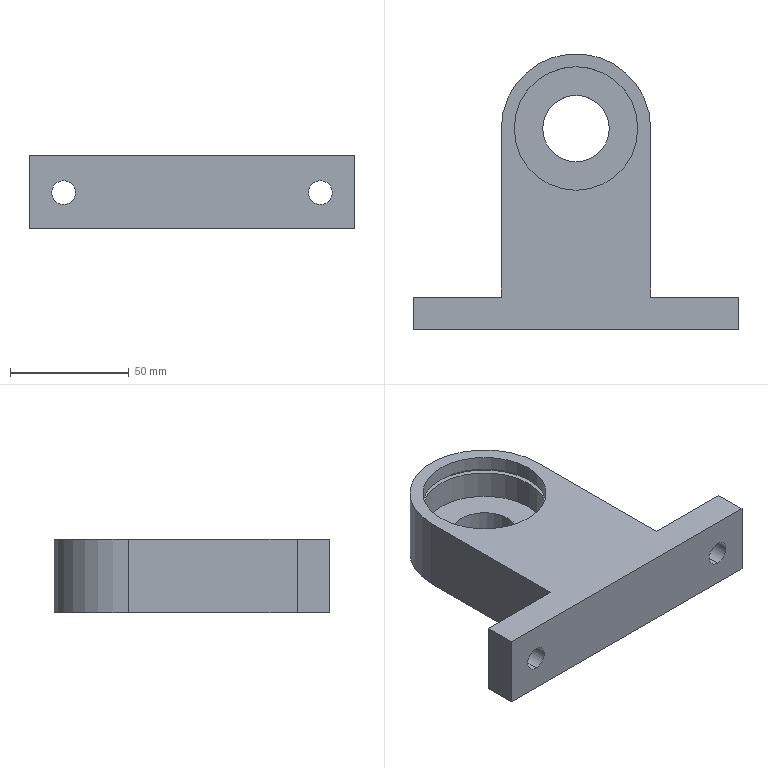Part | SolidWorks | features ICE 3, Cut 1, Extrusion 1 | 1 solid | 25 faces | box 137.013 x 116.006 x 31 mm | volume 192152 mm3 | cylinder 13 | plane 12 | commonest cylinder face diameters 10 x4 52 x4 28 x2 56.2 x2 62.794 x1
STEP:
#1=CARTESIAN_POINT('',(-28.1,0.,25.));
#2=VERTEX_POINT('',#1);
#3=CARTESIAN_POINT('',(28.1,0.,25.));
#4=VERTEX_POINT('',#3);
#5=CARTESIAN_POINT('',(0.,0.,25.));
#6=DIRECTION('',(0.,0.,1.));
#7=DIRECTION('',(1.,0.,0.));
#8=AXIS2_PLACEMENT_3D('',#5,#6,#7);
#9=CIRCLE('',#8,28.1);
#10=EDGE_CURVE('',#2,#4,#9,.T.);
#11=ORIENTED_EDGE('',*,*,#10,.T.);
#12=CARTESIAN_POINT('',(28.1,0.,23.));
#13=VERTEX_POINT('',#12);
#14=CARTESIAN_POINT('',(28.1,0.,25.));
#15=DIRECTION('',(0.,0.,-1.));
#16=VECTOR('',#15,1000.);
#17=LINE('',#14,#16);
#18=EDGE_CURVE('',#4,#13,#17,.T.);
#19=ORIENTED_EDGE('',*,*,#18,.T.);
#20=CARTESIAN_POINT('',(-28.1,0.,23.));
#21=VERTEX_POINT('',#20);
#22=CARTESIAN_POINT('',(0.,0.,23.));
#23=DIRECTION('',(0.,0.,1.));
#24=DIRECTION('',(1.,0.,0.));
#25=AXIS2_PLACEMENT_3D('',#22,#23,#24);
#26=CIRCLE('',#25,28.1);
#27=EDGE_CURVE('',#21,#13,#26,.T.);
#28=ORIENTED_EDGE('',*,*,#27,.F.);
#29=CARTESIAN_POINT('',(-28.1,0.,25.));
#30=DIRECTION('',(0.,0.,-1.));
#31=VECTOR('',#30,1000.);
#32=LINE('',#29,#31);
#33=EDGE_CURVE('',#2,#21,#32,.T.);
#34=ORIENTED_EDGE('',*,*,#33,.F.);
#35=EDGE_LOOP('',(#11,#19,#28,#34));
#36=FACE_OUTER_BOUND('',#35,.T.);
#37=CARTESIAN_POINT('',(0.,0.,25.));
#38=DIRECTION('',(0.,0.,-1.));
#39=DIRECTION('',(-1.,0.,0.));
#40=AXIS2_PLACEMENT_3D('',#37,#38,#39);
#41=CYLINDRICAL_SURFACE('',#40,28.1);
#42=ADVANCED_FACE('',(#36),#41,.F.);
#43=CARTESIAN_POINT('',(26.,0.,25.));
#44=VERTEX_POINT('',#43);
#45=CARTESIAN_POINT('',(-26.,0.,25.));
#46=VERTEX_POINT('',#45);
#47=CARTESIAN_POINT('',(0.,0.,25.));
#48=DIRECTION('',(0.,0.,-1.));
#49=DIRECTION('',(1.,0.,0.));
#50=AXIS2_PLACEMENT_3D('',#47,#48,#49);
#51=CIRCLE('',#50,26.);
#52=EDGE_CURVE('',#44,#46,#51,.T.);
#53=ORIENTED_EDGE('',*,*,#52,.T.);
#54=CARTESIAN_POINT('',(-26.,0.,31.));
#55=VERTEX_POINT('',#54);
#56=CARTESIAN_POINT('',(-26.,0.,11.));
#57=DIRECTION('',(0.,0.,1.));
#58=VECTOR('',#57,1000.);
#59=LINE('',#56,#58);
#60=EDGE_CURVE('',#46,#55,#59,.T.);
#61=ORIENTED_EDGE('',*,*,#60,.T.);
#62=CARTESIAN_POINT('',(26.,0.,31.));
#63=VERTEX_POINT('',#62);
#64=CARTESIAN_POINT('',(0.,0.,31.));
#65=DIRECTION('',(0.,0.,1.));
#66=DIRECTION('',(1.,0.,0.));
#67=AXIS2_PLACEMENT_3D('',#64,#65,#66);
#68=CIRCLE('',#67,26.);
#69=EDGE_CURVE('',#55,#63,#68,.T.);
#70=ORIENTED_EDGE('',*,*,#69,.T.);
#71=CARTESIAN_POINT('',(26.,0.,11.));
#72=DIRECTION('',(0.,0.,1.));
#73=VECTOR('',#72,1000.);
#74=LINE('',#71,#73);
#75=EDGE_CURVE('',#44,#63,#74,.T.);
#76=ORIENTED_EDGE('',*,*,#75,.F.);
#77=EDGE_LOOP('',(#53,#61,#70,#76));
#78=FACE_OUTER_BOUND('',#77,.T.);
#79=CARTESIAN_POINT('',(0.,0.,11.));
#80=DIRECTION('',(0.,0.,1.));
#81=DIRECTION('',(1.,0.,0.));
#82=AXIS2_PLACEMENT_3D('',#79,#80,#81);
#83=CYLINDRICAL_SURFACE('',#82,26.);
#84=ADVANCED_FACE('',(#78),#83,.F.);
#85=CARTESIAN_POINT('',(-54.,-84.609,20.251));
#86=VERTEX_POINT('',#85);
#87=CARTESIAN_POINT('',(-54.,-84.609,10.251));
#88=VERTEX_POINT('',#87);
#89=CARTESIAN_POINT('',(-54.,-84.609,15.251));
#90=DIRECTION('',(0.,-1.,0.));
#91=DIRECTION('',(0.,0.,1.));
#92=AXIS2_PLACEMENT_3D('',#89,#90,#91);
#93=CIRCLE('',#92,5.);
#94=EDGE_CURVE('',#86,#88,#93,.T.);
#95=ORIENTED_EDGE('',*,*,#94,.T.);
#96=CARTESIAN_POINT('',(-54.,-70.889,10.251));
#97=VERTEX_POINT('',#96);
#98=CARTESIAN_POINT('',(-54.,-101.889,10.251));
#99=DIRECTION('',(0.,1.,0.));
#100=VECTOR('',#99,1000.);
#101=LINE('',#98,#100);
#102=EDGE_CURVE('',#88,#97,#101,.T.);
#103=ORIENTED_EDGE('',*,*,#102,.T.);
#104=CARTESIAN_POINT('',(-54.,-70.889,20.251));
#105=VERTEX_POINT('',#104);
#106=CARTESIAN_POINT('',(-54.,-70.889,15.251));
#107=DIRECTION('',(0.,-1.,0.));
#108=DIRECTION('',(0.,0.,1.));
#109=AXIS2_PLACEMENT_3D('',#106,#107,#108);
#110=CIRCLE('',#109,5.);
#111=EDGE_CURVE('',#105,#97,#110,.T.);
#112=ORIENTED_EDGE('',*,*,#111,.F.);
#113=CARTESIAN_POINT('',(-54.,-101.889,20.251));
#114=DIRECTION('',(0.,1.,0.));
#115=VECTOR('',#114,1000.);
#116=LINE('',#113,#115);
#117=EDGE_CURVE('',#86,#105,#116,.T.);
#118=ORIENTED_EDGE('',*,*,#117,.F.);
#119=EDGE_LOOP('',(#95,#103,#112,#118));
#120=FACE_OUTER_BOUND('',#119,.T.);
#121=CARTESIAN_POINT('',(-54.,-101.889,15.251));
#122=DIRECTION('',(0.,1.,0.));
#123=DIRECTION('',(0.,0.,1.));
#124=AXIS2_PLACEMENT_3D('',#121,#122,#123);
#125=CYLINDRICAL_SURFACE('',#124,5.);
#126=ADVANCED_FACE('',(#120),#125,.F.);
#127=CARTESIAN_POINT('',(54.,-84.609,10.251));
#128=VERTEX_POINT('',#127);
#129=CARTESIAN_POINT('',(54.,-84.609,20.251));
#130=VERTEX_POINT('',#129);
#131=CARTESIAN_POINT('',(54.,-84.609,15.251));
#132=DIRECTION('',(0.,1.,0.));
#133=DIRECTION('',(0.,0.,1.));
#134=AXIS2_PLACEMENT_3D('',#131,#132,#133);
#135=CIRCLE('',#134,5.);
#136=EDGE_CURVE('',#128,#130,#135,.T.);
#137=ORIENTED_EDGE('',*,*,#136,.F.);
#138=CARTESIAN_POINT('',(54.,-70.889,10.251));
#139=VERTEX_POINT('',#138);
#140=CARTESIAN_POINT('',(54.,-101.889,10.251));
#141=DIRECTION('',(0.,1.,0.));
#142=VECTOR('',#141,1000.);
#143=LINE('',#140,#142);
#144=EDGE_CURVE('',#128,#139,#143,.T.);
#145=ORIENTED_EDGE('',*,*,#144,.T.);
#146=CARTESIAN_POINT('',(54.,-70.889,20.251));
#147=VERTEX_POINT('',#146);
#148=CARTESIAN_POINT('',(54.,-70.889,15.251));
#149=DIRECTION('',(0.,1.,0.));
#150=DIRECTION('',(0.,0.,1.));
#151=AXIS2_PLACEMENT_3D('',#148,#149,#150);
#152=CIRCLE('',#151,5.);
#153=EDGE_CURVE('',#139,#147,#152,.T.);
#154=ORIENTED_EDGE('',*,*,#153,.T.);
#155=CARTESIAN_POINT('',(54.,-101.889,20.251));
#156=DIRECTION('',(0.,1.,0.));
#157=VECTOR('',#156,1000.);
#158=LINE('',#155,#157);
#159=EDGE_CURVE('',#130,#147,#158,.T.);
#160=ORIENTED_EDGE('',*,*,#159,.F.);
#161=EDGE_LOOP('',(#137,#145,#154,#160));
#162=FACE_OUTER_BOUND('',#161,.T.);
#163=CARTESIAN_POINT('',(54.,-101.889,15.251));
#164=DIRECTION('',(0.,1.,0.));
#165=DIRECTION('',(0.,0.,1.));
#166=AXIS2_PLACEMENT_3D('',#163,#164,#165);
#167=CYLINDRICAL_SURFACE('',#166,5.);
#168=ADVANCED_FACE('',(#162),#167,.F.);
#169=CARTESIAN_POINT('',(14.,0.,11.));
#170=VERTEX_POINT('',#169);
#171=CARTESIAN_POINT('',(-14.,0.,11.));
#172=VERTEX_POINT('',#171);
#173=CARTESIAN_POINT('',(0.,0.,11.));
#174=DIRECTION('',(0.,0.,-1.));
#175=DIRECTION('',(1.,0.,0.));
#176=AXIS2_PLACEMENT_3D('',#173,#174,#175);
#177=CIRCLE('',#176,14.);
#178=EDGE_CURVE('',#170,#172,#177,.T.);
#179=ORIENTED_EDGE('',*,*,#178,.F.);
#180=CARTESIAN_POINT('',(14.,0.,0.));
#181=VERTEX_POINT('',#180);
#182=CARTESIAN_POINT('',(14.,0.,31.));
#183=DIRECTION('',(0.,0.,-1.));
#184=VECTOR('',#183,1000.);
#185=LINE('',#182,#184);
#186=EDGE_CURVE('',#170,#181,#185,.T.);
#187=ORIENTED_EDGE('',*,*,#186,.T.);
#188=CARTESIAN_POINT('',(-14.,0.,0.));
#189=VERTEX_POINT('',#188);
#190=CARTESIAN_POINT('',(0.,0.,0.));
#191=DIRECTION('',(0.,0.,-1.));
#192=DIRECTION('',(-1.,0.,0.));
#193=AXIS2_PLACEMENT_3D('',#190,#191,#192);
#194=CIRCLE('',#193,14.);
#195=EDGE_CURVE('',#181,#189,#194,.T.);
#196=ORIENTED_EDGE('',*,*,#195,.T.);
#197=CARTESIAN_POINT('',(-14.,0.,31.));
#198=DIRECTION('',(0.,0.,-1.));
#199=VECTOR('',#198,1000.);
#200=LINE('',#197,#199);
#201=EDGE_CURVE('',#172,#189,#200,.T.);
#202=ORIENTED_EDGE('',*,*,#201,.F.);
#203=EDGE_LOOP('',(#179,#187,#196,#202));
#204=FACE_OUTER_BOUND('',#203,.T.);
#205=CARTESIAN_POINT('',(0.,0.,31.));
#206=DIRECTION('',(0.,0.,-1.));
#207=DIRECTION('',(-1.,0.,0.));
#208=AXIS2_PLACEMENT_3D('',#205,#206,#207);
#209=CYLINDRICAL_SURFACE('',#208,14.);
#210=ADVANCED_FACE('',(#204),#209,.F.);
#211=CARTESIAN_POINT('',(-26.,0.,11.));
#212=VERTEX_POINT('',#211);
#213=CARTESIAN_POINT('',(26.,0.,11.));
#214=VERTEX_POINT('',#213);
#215=CARTESIAN_POINT('',(0.,0.,11.));
#216=DIRECTION('',(0.,0.,1.));
#217=DIRECTION('',(1.,0.,0.));
#218=AXIS2_PLACEMENT_3D('',#215,#216,#217);
#219=CIRCLE('',#218,26.);
#220=EDGE_CURVE('',#212,#214,#219,.T.);
#221=ORIENTED_EDGE('',*,*,#220,.F.);
#222=CARTESIAN_POINT('',(-26.,0.,23.));
#223=VERTEX_POINT('',#222);
#224=CARTESIAN_POINT('',(-26.,0.,11.));
#225=DIRECTION('',(0.,0.,1.));
#226=VECTOR('',#225,1000.);
#227=LINE('',#224,#226);
#228=EDGE_CURVE('',#212,#223,#227,.T.);
#229=ORIENTED_EDGE('',*,*,#228,.T.);
#230=CARTESIAN_POINT('',(26.,0.,23.));
#231=VERTEX_POINT('',#230);
#232=CARTESIAN_POINT('',(0.,0.,23.));
#233=DIRECTION('',(0.,0.,-1.));
#234=DIRECTION('',(1.,0.,0.));
#235=AXIS2_PLACEMENT_3D('',#232,#233,#234);
#236=CIRCLE('',#235,26.);
#237=EDGE_CURVE('',#231,#223,#236,.T.);
#238=ORIENTED_EDGE('',*,*,#237,.F.);
#239=CARTESIAN_POINT('',(26.,0.,11.));
#240=DIRECTION('',(0.,0.,1.));
#241=VECTOR('',#240,1000.);
#242=LINE('',#239,#241);
#243=EDGE_CURVE('',#214,#231,#242,.T.);
#244=ORIENTED_EDGE('',*,*,#243,.F.);
#245=EDGE_LOOP('',(#221,#229,#238,#244));
#246=FACE_OUTER_BOUND('',#245,.T.);
#247=CARTESIAN_POINT('',(0.,0.,11.));
#248=DIRECTION('',(0.,0.,1.));
#249=DIRECTION('',(1.,0.,0.));
#250=AXIS2_PLACEMENT_3D('',#247,#248,#249);
#251=CYLINDRICAL_SURFACE('',#250,26.);
#252=ADVANCED_FACE('',(#246),#251,.F.);
#253=ORIENTED_EDGE('',*,*,#228,.F.);
#254=CARTESIAN_POINT('',(0.,0.,11.));
#255=DIRECTION('',(0.,0.,1.));
#256=DIRECTION('',(1.,0.,0.));
#257=AXIS2_PLACEMENT_3D('',#254,#255,#256);
#258=CIRCLE('',#257,26.);
#259=EDGE_CURVE('',#214,#212,#258,.T.);
#260=ORIENTED_EDGE('',*,*,#259,.F.);
#261=ORIENTED_EDGE('',*,*,#243,.T.);
#262=CARTESIAN_POINT('',(0.,0.,23.));
#263=DIRECTION('',(0.,0.,-1.));
#264=DIRECTION('',(1.,0.,0.));
#265=AXIS2_PLACEMENT_3D('',#262,#263,#264);
#266=CIRCLE('',#265,26.);
#267=EDGE_CURVE('',#223,#231,#266,.T.);
#268=ORIENTED_EDGE('',*,*,#267,.F.);
#269=EDGE_LOOP('',(#253,#260,#261,#268));
#270=FACE_OUTER_BOUND('',#269,.T.);
#271=CARTESIAN_POINT('',(0.,0.,11.));
#272=DIRECTION('',(0.,0.,1.));
#273=DIRECTION('',(1.,0.,0.));
#274=AXIS2_PLACEMENT_3D('',#271,#272,#273);
#275=CYLINDRICAL_SURFACE('',#274,26.);
#276=ADVANCED_FACE('',(#270),#275,.F.);
#277=ORIENTED_EDGE('',*,*,#186,.F.);
#278=CARTESIAN_POINT('',(0.,0.,11.));
#279=DIRECTION('',(0.,0.,-1.));
#280=DIRECTION('',(1.,0.,0.));
#281=AXIS2_PLACEMENT_3D('',#278,#279,#280);
#282=CIRCLE('',#281,14.);
#283=EDGE_CURVE('',#172,#170,#282,.T.);
#284=ORIENTED_EDGE('',*,*,#283,.F.);
#285=ORIENTED_EDGE('',*,*,#201,.T.);
#286=CARTESIAN_POINT('',(0.,0.,0.));
#287=DIRECTION('',(0.,0.,-1.));
#288=DIRECTION('',(-1.,0.,0.));
#289=AXIS2_PLACEMENT_3D('',#286,#287,#288);
#290=CIRCLE('',#289,14.);
#291=EDGE_CURVE('',#189,#181,#290,.T.);
#292=ORIENTED_EDGE('',*,*,#291,.T.);
#293=EDGE_LOOP('',(#277,#284,#285,#292));
#294=FACE_OUTER_BOUND('',#293,.T.);
#295=CARTESIAN_POINT('',(0.,0.,31.));
#296=DIRECTION('',(0.,0.,-1.));
#297=DIRECTION('',(-1.,0.,0.));
#298=AXIS2_PLACEMENT_3D('',#295,#296,#297);
#299=CYLINDRICAL_SURFACE('',#298,14.);
#300=ADVANCED_FACE('',(#294),#299,.F.);
#301=CARTESIAN_POINT('',(-68.507,-84.609,0.));
#302=VERTEX_POINT('',#301);
#303=CARTESIAN_POINT('',(68.507,-84.609,0.));
#304=VERTEX_POINT('',#303);
#305=CARTESIAN_POINT('',(0.,-84.609,0.));
#306=DIRECTION('',(1.,0.,0.));
#307=VECTOR('',#306,1000.);
#308=LINE('',#305,#307);
#309=EDGE_CURVE('',#302,#304,#308,.T.);
#310=ORIENTED_EDGE('',*,*,#309,.T.);
#311=CARTESIAN_POINT('',(68.507,-84.609,31.));
#312=VERTEX_POINT('',#311);
#313=CARTESIAN_POINT('',(68.507,-84.609,31.));
#314=DIRECTION('',(0.,0.,-1.));
#315=VECTOR('',#314,1000.);
#316=LINE('',#313,#315);
#317=EDGE_CURVE('',#312,#304,#316,.T.);
#318=ORIENTED_EDGE('',*,*,#317,.F.);
#319=CARTESIAN_POINT('',(-68.507,-84.609,31.));
#320=VERTEX_POINT('',#319);
#321=CARTESIAN_POINT('',(0.,-84.609,31.));
#322=DIRECTION('',(1.,0.,0.));
#323=VECTOR('',#322,1000.);
#324=LINE('',#321,#323);
#325=EDGE_CURVE('',#320,#312,#324,.T.);
#326=ORIENTED_EDGE('',*,*,#325,.F.);
#327=CARTESIAN_POINT('',(-68.507,-84.609,31.));
#328=DIRECTION('',(0.,0.,-1.));
#329=VECTOR('',#328,1000.);
#330=LINE('',#327,#329);
#331=EDGE_CURVE('',#320,#302,#330,.T.);
#332=ORIENTED_EDGE('',*,*,#331,.T.);
#333=EDGE_LOOP('',(#310,#318,#326,#332));
#334=FACE_OUTER_BOUND('',#333,.T.);
#335=ORIENTED_EDGE('',*,*,#94,.F.);
#336=CARTESIAN_POINT('',(-54.,-84.609,15.251));
#337=DIRECTION('',(0.,-1.,0.));
#338=DIRECTION('',(0.,0.,1.));
#339=AXIS2_PLACEMENT_3D('',#336,#337,#338);
#340=CIRCLE('',#339,5.);
#341=EDGE_CURVE('',#88,#86,#340,.T.);
#342=ORIENTED_EDGE('',*,*,#341,.F.);
#343=EDGE_LOOP('',(#335,#342));
#344=FACE_BOUND('',#343,.T.);
#345=CARTESIAN_POINT('',(54.,-84.609,15.251));
#346=DIRECTION('',(0.,1.,0.));
#347=DIRECTION('',(0.,0.,1.));
#348=AXIS2_PLACEMENT_3D('',#345,#346,#347);
#349=CIRCLE('',#348,5.);
#350=EDGE_CURVE('',#130,#128,#349,.T.);
#351=ORIENTED_EDGE('',*,*,#350,.T.);
#352=ORIENTED_EDGE('',*,*,#136,.T.);
#353=EDGE_LOOP('',(#351,#352));
#354=FACE_BOUND('',#353,.T.);
#355=CARTESIAN_POINT('',(0.,-84.609,31.));
#356=DIRECTION('',(0.,1.,0.));
#357=DIRECTION('',(0.,0.,1.));
#358=AXIS2_PLACEMENT_3D('',#355,#356,#357);
#359=PLANE('',#358);
#360=ADVANCED_FACE('',(#334,#344,#354),#359,.F.);
#361=CARTESIAN_POINT('',(31.397,0.,0.));
#362=VERTEX_POINT('',#361);
#363=CARTESIAN_POINT('',(-31.397,0.,0.));
#364=VERTEX_POINT('',#363);
#365=CARTESIAN_POINT('',(0.,0.,0.));
#366=DIRECTION('',(0.,0.,1.));
#367=DIRECTION('',(1.,0.,0.));
#368=AXIS2_PLACEMENT_3D('',#365,#366,#367);
#369=CIRCLE('',#368,31.397);
#370=EDGE_CURVE('',#362,#364,#369,.T.);
#371=ORIENTED_EDGE('',*,*,#370,.T.);
#372=CARTESIAN_POINT('',(-31.397,0.,31.));
#373=VERTEX_POINT('',#372);
#374=CARTESIAN_POINT('',(-31.397,0.,31.));
#375=DIRECTION('',(0.,0.,-1.));
#376=VECTOR('',#375,1000.);
#377=LINE('',#374,#376);
#378=EDGE_CURVE('',#373,#364,#377,.T.);
#379=ORIENTED_EDGE('',*,*,#378,.F.);
#380=CARTESIAN_POINT('',(31.397,0.,31.));
#381=VERTEX_POINT('',#380);
#382=CARTESIAN_POINT('',(0.,0.,31.));
#383=DIRECTION('',(0.,0.,1.));
#384=DIRECTION('',(1.,0.,0.));
#385=AXIS2_PLACEMENT_3D('',#382,#383,#384);
#386=CIRCLE('',#385,31.397);
#387=EDGE_CURVE('',#381,#373,#386,.T.);
#388=ORIENTED_EDGE('',*,*,#387,.F.);
#389=CARTESIAN_POINT('',(31.397,0.,31.));
#390=DIRECTION('',(0.,0.,-1.));
#391=VECTOR('',#390,1000.);
#392=LINE('',#389,#391);
#393=EDGE_CURVE('',#381,#362,#392,.T.);
#394=ORIENTED_EDGE('',*,*,#393,.T.);
#395=EDGE_LOOP('',(#371,#379,#388,#394));
#396=FACE_OUTER_BOUND('',#395,.T.);
#397=CARTESIAN_POINT('',(0.,0.,31.));
#398=DIRECTION('',(0.,0.,-1.));
#399=DIRECTION('',(-1.,0.,0.));
#400=AXIS2_PLACEMENT_3D('',#397,#398,#399);
#401=CYLINDRICAL_SURFACE('',#400,31.397);
#402=ADVANCED_FACE('',(#396),#401,.T.);
#403=CARTESIAN_POINT('',(-31.397,-70.889,0.));
#404=VERTEX_POINT('',#403);
#405=CARTESIAN_POINT('',(-31.397,0.,0.));
#406=DIRECTION('',(0.,-1.,0.));
#407=VECTOR('',#406,1000.);
#408=LINE('',#405,#407);
#409=EDGE_CURVE('',#364,#404,#408,.T.);
#410=ORIENTED_EDGE('',*,*,#409,.T.);
#411=CARTESIAN_POINT('',(-31.397,-70.889,31.));
#412=VERTEX_POINT('',#411);
#413=CARTESIAN_POINT('',(-31.397,-70.889,31.));
#414=DIRECTION('',(0.,0.,-1.));
#415=VECTOR('',#414,1000.);
#416=LINE('',#413,#415);
#417=EDGE_CURVE('',#412,#404,#416,.T.);
#418=ORIENTED_EDGE('',*,*,#417,.F.);
#419=CARTESIAN_POINT('',(-31.397,0.,31.));
#420=DIRECTION('',(0.,-1.,0.));
#421=VECTOR('',#420,1000.);
#422=LINE('',#419,#421);
#423=EDGE_CURVE('',#373,#412,#422,.T.);
#424=ORIENTED_EDGE('',*,*,#423,.F.);
#425=ORIENTED_EDGE('',*,*,#378,.T.);
#426=EDGE_LOOP('',(#410,#418,#424,#425));
#427=FACE_OUTER_BOUND('',#426,.T.);
#428=CARTESIAN_POINT('',(-31.397,0.,31.));
#429=DIRECTION('',(1.,0.,0.));
#430=DIRECTION('',(0.,0.,-1.));
#431=AXIS2_PLACEMENT_3D('',#428,#429,#430);
#432=PLANE('',#431);
#433=ADVANCED_FACE('',(#427),#432,.F.);
#434=ORIENTED_EDGE('',*,*,#111,.T.);
#435=CARTESIAN_POINT('',(-54.,-70.889,15.251));
#436=DIRECTION('',(0.,-1.,0.));
#437=DIRECTION('',(0.,0.,1.));
#438=AXIS2_PLACEMENT_3D('',#435,#436,#437);
#439=CIRCLE('',#438,5.);
#440=EDGE_CURVE('',#97,#105,#439,.T.);
#441=ORIENTED_EDGE('',*,*,#440,.T.);
#442=EDGE_LOOP('',(#434,#441));
#443=FACE_BOUND('',#442,.T.);
#444=CARTESIAN_POINT('',(-68.507,-70.889,0.));
#445=VERTEX_POINT('',#444);
#446=CARTESIAN_POINT('',(0.,-70.889,0.));
#447=DIRECTION('',(-1.,0.,0.));
#448=VECTOR('',#447,1000.);
#449=LINE('',#446,#448);
#450=EDGE_CURVE('',#404,#445,#449,.T.);
#451=ORIENTED_EDGE('',*,*,#450,.T.);
#452=CARTESIAN_POINT('',(-68.507,-70.889,31.));
#453=VERTEX_POINT('',#452);
#454=CARTESIAN_POINT('',(-68.507,-70.889,31.));
#455=DIRECTION('',(0.,0.,-1.));
#456=VECTOR('',#455,1000.);
#457=LINE('',#454,#456);
#458=EDGE_CURVE('',#453,#445,#457,.T.);
#459=ORIENTED_EDGE('',*,*,#458,.F.);
#460=CARTESIAN_POINT('',(0.,-70.889,31.));
#461=DIRECTION('',(-1.,0.,0.));
#462=VECTOR('',#461,1000.);
#463=LINE('',#460,#462);
#464=EDGE_CURVE('',#412,#453,#463,.T.);
#465=ORIENTED_EDGE('',*,*,#464,.F.);
#466=ORIENTED_EDGE('',*,*,#417,.T.);
#467=EDGE_LOOP('',(#451,#459,#465,#466));
#468=FACE_OUTER_BOUND('',#467,.T.);
#469=CARTESIAN_POINT('',(0.,-70.889,31.));
#470=DIRECTION('',(0.,-1.,0.));
#471=DIRECTION('',(0.,0.,-1.));
#472=AXIS2_PLACEMENT_3D('',#469,#470,#471);
#473=PLANE('',#472);
#474=ADVANCED_FACE('',(#443,#468),#473,.F.);
#475=CARTESIAN_POINT('',(-68.507,0.,0.));
#476=DIRECTION('',(0.,-1.,0.));
#477=VECTOR('',#476,1000.);
#478=LINE('',#475,#477);
#479=EDGE_CURVE('',#445,#302,#478,.T.);
#480=ORIENTED_EDGE('',*,*,#479,.T.);
#481=ORIENTED_EDGE('',*,*,#331,.F.);
#482=CARTESIAN_POINT('',(-68.507,0.,31.));
#483=DIRECTION('',(0.,-1.,0.));
#484=VECTOR('',#483,1000.);
#485=LINE('',#482,#484);
#486=EDGE_CURVE('',#453,#320,#485,.T.);
#487=ORIENTED_EDGE('',*,*,#486,.F.);
#488=ORIENTED_EDGE('',*,*,#458,.T.);
#489=EDGE_LOOP('',(#480,#481,#487,#488));
#490=FACE_OUTER_BOUND('',#489,.T.);
#491=CARTESIAN_POINT('',(-68.507,0.,31.));
#492=DIRECTION('',(1.,0.,0.));
#493=DIRECTION('',(0.,0.,-1.));
#494=AXIS2_PLACEMENT_3D('',#491,#492,#493);
#495=PLANE('',#494);
#496=ADVANCED_FACE('',(#490),#495,.F.);
#497=CARTESIAN_POINT('',(68.507,-70.889,0.));
#498=VERTEX_POINT('',#497);
#499=CARTESIAN_POINT('',(68.507,0.,0.));
#500=DIRECTION('',(0.,-1.,0.));
#501=VECTOR('',#500,1000.);
#502=LINE('',#499,#501);
#503=EDGE_CURVE('',#498,#304,#502,.T.);
#504=ORIENTED_EDGE('',*,*,#503,.F.);
#505=CARTESIAN_POINT('',(68.507,-70.889,31.));
#506=VERTEX_POINT('',#505);
#507=CARTESIAN_POINT('',(68.507,-70.889,31.));
#508=DIRECTION('',(0.,0.,-1.));
#509=VECTOR('',#508,1000.);
#510=LINE('',#507,#509);
#511=EDGE_CURVE('',#506,#498,#510,.T.);
#512=ORIENTED_EDGE('',*,*,#511,.F.);
#513=CARTESIAN_POINT('',(68.507,0.,31.));
#514=DIRECTION('',(0.,-1.,0.));
#515=VECTOR('',#514,1000.);
#516=LINE('',#513,#515);
#517=EDGE_CURVE('',#506,#312,#516,.T.);
#518=ORIENTED_EDGE('',*,*,#517,.T.);
#519=ORIENTED_EDGE('',*,*,#317,.T.);
#520=EDGE_LOOP('',(#504,#512,#518,#519));
#521=FACE_OUTER_BOUND('',#520,.T.);
#522=CARTESIAN_POINT('',(68.507,0.,31.));
#523=DIRECTION('',(1.,0.,0.));
#524=DIRECTION('',(0.,0.,-1.));
#525=AXIS2_PLACEMENT_3D('',#522,#523,#524);
#526=PLANE('',#525);
#527=ADVANCED_FACE('',(#521),#526,.T.);
#528=CARTESIAN_POINT('',(54.,-70.889,15.251));
#529=DIRECTION('',(0.,1.,0.));
#530=DIRECTION('',(0.,0.,1.));
#531=AXIS2_PLACEMENT_3D('',#528,#529,#530);
#532=CIRCLE('',#531,5.);
#533=EDGE_CURVE('',#147,#139,#532,.T.);
#534=ORIENTED_EDGE('',*,*,#533,.F.);
#535=ORIENTED_EDGE('',*,*,#153,.F.);
#536=EDGE_LOOP('',(#534,#535));
#537=FACE_BOUND('',#536,.T.);
#538=CARTESIAN_POINT('',(31.397,-70.889,0.));
#539=VERTEX_POINT('',#538);
#540=CARTESIAN_POINT('',(0.,-70.889,0.));
#541=DIRECTION('',(1.,0.,0.));
#542=VECTOR('',#541,1000.);
#543=LINE('',#540,#542);
#544=EDGE_CURVE('',#539,#498,#543,.T.);
#545=ORIENTED_EDGE('',*,*,#544,.F.);
#546=CARTESIAN_POINT('',(31.397,-70.889,31.));
#547=VERTEX_POINT('',#546);
#548=CARTESIAN_POINT('',(31.397,-70.889,31.));
#549=DIRECTION('',(0.,0.,-1.));
#550=VECTOR('',#549,1000.);
#551=LINE('',#548,#550);
#552=EDGE_CURVE('',#547,#539,#551,.T.);
#553=ORIENTED_EDGE('',*,*,#552,.F.);
#554=CARTESIAN_POINT('',(0.,-70.889,31.));
#555=DIRECTION('',(1.,0.,0.));
#556=VECTOR('',#555,1000.);
#557=LINE('',#554,#556);
#558=EDGE_CURVE('',#547,#506,#557,.T.);
#559=ORIENTED_EDGE('',*,*,#558,.T.);
#560=ORIENTED_EDGE('',*,*,#511,.T.);
#561=EDGE_LOOP('',(#545,#553,#559,#560));
#562=FACE_OUTER_BOUND('',#561,.T.);
#563=CARTESIAN_POINT('',(0.,-70.889,31.));
#564=DIRECTION('',(0.,1.,0.));
#565=DIRECTION('',(0.,0.,1.));
#566=AXIS2_PLACEMENT_3D('',#563,#564,#565);
#567=PLANE('',#566);
#568=ADVANCED_FACE('',(#537,#562),#567,.T.);
#569=CARTESIAN_POINT('',(31.397,0.,0.));
#570=DIRECTION('',(0.,-1.,0.));
#571=VECTOR('',#570,1000.);
#572=LINE('',#569,#571);
#573=EDGE_CURVE('',#362,#539,#572,.T.);
#574=ORIENTED_EDGE('',*,*,#573,.F.);
#575=ORIENTED_EDGE('',*,*,#393,.F.);
#576=CARTESIAN_POINT('',(31.397,0.,31.));
#577=DIRECTION('',(0.,-1.,0.));
#578=VECTOR('',#577,1000.);
#579=LINE('',#576,#578);
#580=EDGE_CURVE('',#381,#547,#579,.T.);
#581=ORIENTED_EDGE('',*,*,#580,.T.);
#582=ORIENTED_EDGE('',*,*,#552,.T.);
#583=EDGE_LOOP('',(#574,#575,#581,#582));
#584=FACE_OUTER_BOUND('',#583,.T.);
#585=CARTESIAN_POINT('',(31.397,0.,31.));
#586=DIRECTION('',(1.,0.,0.));
#587=DIRECTION('',(0.,0.,-1.));
#588=AXIS2_PLACEMENT_3D('',#585,#586,#587);
#589=PLANE('',#588);
#590=ADVANCED_FACE('',(#584),#589,.T.);
#591=CARTESIAN_POINT('',(0.,0.,31.));
#592=DIRECTION('',(0.,0.,1.));
#593=DIRECTION('',(1.,0.,0.));
#594=AXIS2_PLACEMENT_3D('',#591,#592,#593);
#595=CIRCLE('',#594,26.);
#596=EDGE_CURVE('',#63,#55,#595,.T.);
#597=ORIENTED_EDGE('',*,*,#596,.F.);
#598=ORIENTED_EDGE('',*,*,#69,.F.);
#599=EDGE_LOOP('',(#597,#598));
#600=FACE_BOUND('',#599,.T.);
#601=ORIENTED_EDGE('',*,*,#387,.T.);
#602=ORIENTED_EDGE('',*,*,#423,.T.);
#603=ORIENTED_EDGE('',*,*,#464,.T.);
#604=ORIENTED_EDGE('',*,*,#486,.T.);
#605=ORIENTED_EDGE('',*,*,#325,.T.);
#606=ORIENTED_EDGE('',*,*,#517,.F.);
#607=ORIENTED_EDGE('',*,*,#558,.F.);
#608=ORIENTED_EDGE('',*,*,#580,.F.);
#609=EDGE_LOOP('',(#601,#602,#603,#604,#605,#606,#607,#608));
#610=FACE_OUTER_BOUND('',#609,.T.);
#611=CARTESIAN_POINT('',(0.,0.,31.));
#612=DIRECTION('',(0.,0.,1.));
#613=DIRECTION('',(1.,0.,0.));
#614=AXIS2_PLACEMENT_3D('',#611,#612,#613);
#615=PLANE('',#614);
#616=ADVANCED_FACE('',(#600,#610),#615,.T.);
#617=ORIENTED_EDGE('',*,*,#291,.F.);
#618=ORIENTED_EDGE('',*,*,#195,.F.);
#619=EDGE_LOOP('',(#617,#618));
#620=FACE_BOUND('',#619,.T.);
#621=ORIENTED_EDGE('',*,*,#370,.F.);
#622=ORIENTED_EDGE('',*,*,#573,.T.);
#623=ORIENTED_EDGE('',*,*,#544,.T.);
#624=ORIENTED_EDGE('',*,*,#503,.T.);
#625=ORIENTED_EDGE('',*,*,#309,.F.);
#626=ORIENTED_EDGE('',*,*,#479,.F.);
#627=ORIENTED_EDGE('',*,*,#450,.F.);
#628=ORIENTED_EDGE('',*,*,#409,.F.);
#629=EDGE_LOOP('',(#621,#622,#623,#624,#625,#626,#627,#628));
#630=FACE_OUTER_BOUND('',#629,.T.);
#631=CARTESIAN_POINT('',(0.,0.,0.));
#632=DIRECTION('',(0.,0.,1.));
#633=DIRECTION('',(1.,0.,0.));
#634=AXIS2_PLACEMENT_3D('',#631,#632,#633);
#635=PLANE('',#634);
#636=ADVANCED_FACE('',(#620,#630),#635,.F.);
#637=ORIENTED_EDGE('',*,*,#144,.F.);
#638=ORIENTED_EDGE('',*,*,#350,.F.);
#639=ORIENTED_EDGE('',*,*,#159,.T.);
#640=ORIENTED_EDGE('',*,*,#533,.T.);
#641=EDGE_LOOP('',(#637,#638,#639,#640));
#642=FACE_OUTER_BOUND('',#641,.T.);
#643=CARTESIAN_POINT('',(54.,-101.889,15.251));
#644=DIRECTION('',(0.,1.,0.));
#645=DIRECTION('',(0.,0.,1.));
#646=AXIS2_PLACEMENT_3D('',#643,#644,#645);
#647=CYLINDRICAL_SURFACE('',#646,5.);
#648=ADVANCED_FACE('',(#642),#647,.F.);
#649=ORIENTED_EDGE('',*,*,#102,.F.);
#650=ORIENTED_EDGE('',*,*,#341,.T.);
#651=ORIENTED_EDGE('',*,*,#117,.T.);
#652=ORIENTED_EDGE('',*,*,#440,.F.);
#653=EDGE_LOOP('',(#649,#650,#651,#652));
#654=FACE_OUTER_BOUND('',#653,.T.);
#655=CARTESIAN_POINT('',(-54.,-101.889,15.251));
#656=DIRECTION('',(0.,1.,0.));
#657=DIRECTION('',(0.,0.,1.));
#658=AXIS2_PLACEMENT_3D('',#655,#656,#657);
#659=CYLINDRICAL_SURFACE('',#658,5.);
#660=ADVANCED_FACE('',(#654),#659,.F.);
#661=ORIENTED_EDGE('',*,*,#259,.T.);
#662=ORIENTED_EDGE('',*,*,#220,.T.);
#663=EDGE_LOOP('',(#661,#662));
#664=FACE_OUTER_BOUND('',#663,.T.);
#665=ORIENTED_EDGE('',*,*,#283,.T.);
#666=ORIENTED_EDGE('',*,*,#178,.T.);
#667=EDGE_LOOP('',(#665,#666));
#668=FACE_BOUND('',#667,.T.);
#669=CARTESIAN_POINT('',(0.,0.,11.));
#670=DIRECTION('',(0.,0.,1.));
#671=DIRECTION('',(1.,0.,0.));
#672=AXIS2_PLACEMENT_3D('',#669,#670,#671);
#673=PLANE('',#672);
#674=ADVANCED_FACE('',(#664,#668),#673,.T.);
#675=ORIENTED_EDGE('',*,*,#60,.F.);
#676=CARTESIAN_POINT('',(0.,0.,25.));
#677=DIRECTION('',(0.,0.,-1.));
#678=DIRECTION('',(1.,0.,0.));
#679=AXIS2_PLACEMENT_3D('',#676,#677,#678);
#680=CIRCLE('',#679,26.);
#681=EDGE_CURVE('',#46,#44,#680,.T.);
#682=ORIENTED_EDGE('',*,*,#681,.T.);
#683=ORIENTED_EDGE('',*,*,#75,.T.);
#684=ORIENTED_EDGE('',*,*,#596,.T.);
#685=EDGE_LOOP('',(#675,#682,#683,#684));
#686=FACE_OUTER_BOUND('',#685,.T.);
#687=CARTESIAN_POINT('',(0.,0.,11.));
#688=DIRECTION('',(0.,0.,1.));
#689=DIRECTION('',(1.,0.,0.));
#690=AXIS2_PLACEMENT_3D('',#687,#688,#689);
#691=CYLINDRICAL_SURFACE('',#690,26.);
#692=ADVANCED_FACE('',(#686),#691,.F.);
#693=ORIENTED_EDGE('',*,*,#10,.F.);
#694=CARTESIAN_POINT('',(0.,0.,25.));
#695=DIRECTION('',(0.,0.,1.));
#696=DIRECTION('',(1.,0.,0.));
#697=AXIS2_PLACEMENT_3D('',#694,#695,#696);
#698=CIRCLE('',#697,28.1);
#699=EDGE_CURVE('',#4,#2,#698,.T.);
#700=ORIENTED_EDGE('',*,*,#699,.F.);
#701=EDGE_LOOP('',(#693,#700));
#702=FACE_OUTER_BOUND('',#701,.T.);
#703=ORIENTED_EDGE('',*,*,#52,.F.);
#704=ORIENTED_EDGE('',*,*,#681,.F.);
#705=EDGE_LOOP('',(#703,#704));
#706=FACE_BOUND('',#705,.T.);
#707=CARTESIAN_POINT('',(0.,0.,25.));
#708=DIRECTION('',(0.,0.,1.));
#709=DIRECTION('',(1.,0.,0.));
#710=AXIS2_PLACEMENT_3D('',#707,#708,#709);
#711=PLANE('',#710);
#712=ADVANCED_FACE('',(#702,#706),#711,.F.);
#713=ORIENTED_EDGE('',*,*,#27,.T.);
#714=CARTESIAN_POINT('',(0.,0.,23.));
#715=DIRECTION('',(0.,0.,1.));
#716=DIRECTION('',(1.,0.,0.));
#717=AXIS2_PLACEMENT_3D('',#714,#715,#716);
#718=CIRCLE('',#717,28.1);
#719=EDGE_CURVE('',#13,#21,#718,.T.);
#720=ORIENTED_EDGE('',*,*,#719,.T.);
#721=EDGE_LOOP('',(#713,#720));
#722=FACE_OUTER_BOUND('',#721,.T.);
#723=ORIENTED_EDGE('',*,*,#237,.T.);
#724=ORIENTED_EDGE('',*,*,#267,.T.);
#725=EDGE_LOOP('',(#723,#724));
#726=FACE_BOUND('',#725,.T.);
#727=CARTESIAN_POINT('',(0.,0.,23.));
#728=DIRECTION('',(0.,0.,1.));
#729=DIRECTION('',(1.,0.,0.));
#730=AXIS2_PLACEMENT_3D('',#727,#728,#729);
#731=PLANE('',#730);
#732=ADVANCED_FACE('',(#722,#726),#731,.T.);
#733=ORIENTED_EDGE('',*,*,#18,.F.);
#734=ORIENTED_EDGE('',*,*,#699,.T.);
#735=ORIENTED_EDGE('',*,*,#33,.T.);
#736=ORIENTED_EDGE('',*,*,#719,.F.);
#737=EDGE_LOOP('',(#733,#734,#735,#736));
#738=FACE_OUTER_BOUND('',#737,.T.);
#739=CARTESIAN_POINT('',(0.,0.,25.));
#740=DIRECTION('',(0.,0.,-1.));
#741=DIRECTION('',(-1.,0.,0.));
#742=AXIS2_PLACEMENT_3D('',#739,#740,#741);
#743=CYLINDRICAL_SURFACE('',#742,28.1);
#744=ADVANCED_FACE('',(#738),#743,.F.);
#745=CLOSED_SHELL('',(#42,#84,#126,#168,#210,#252,#276,#300,#360,#402,#433,#474,#496,#527,#568,#590,#616,#636,#648,#660,#674,#692,#712,#732,#744));
#746=MANIFOLD_SOLID_BREP('',#745);
#747=CARTESIAN_POINT('',(0.,0.,0.));
#748=DIRECTION('',(0.,0.,1.));
#749=DIRECTION('',(1.,0.,0.));
#750=AXIS2_PLACEMENT_3D('',#747,#748,#749);
#751=(LENGTH_UNIT()NAMED_UNIT(*)SI_UNIT(.MILLI.,.METRE.));
#752=UNCERTAINTY_MEASURE_WITH_UNIT(LENGTH_MEASURE(0.00001),#751,'','');
#753=(NAMED_UNIT(*)PLANE_ANGLE_UNIT()SI_UNIT($,.RADIAN.));
#754=(NAMED_UNIT(*)SI_UNIT($,.STERADIAN.)SOLID_ANGLE_UNIT());
#755=(GEOMETRIC_REPRESENTATION_CONTEXT(3)GLOBAL_UNCERTAINTY_ASSIGNED_CONTEXT((#752))GLOBAL_UNIT_ASSIGNED_CONTEXT((#751,#753,#754))REPRESENTATION_CONTEXT('',''));
#756=ADVANCED_BREP_SHAPE_REPRESENTATION('',(#746,#750),#755);